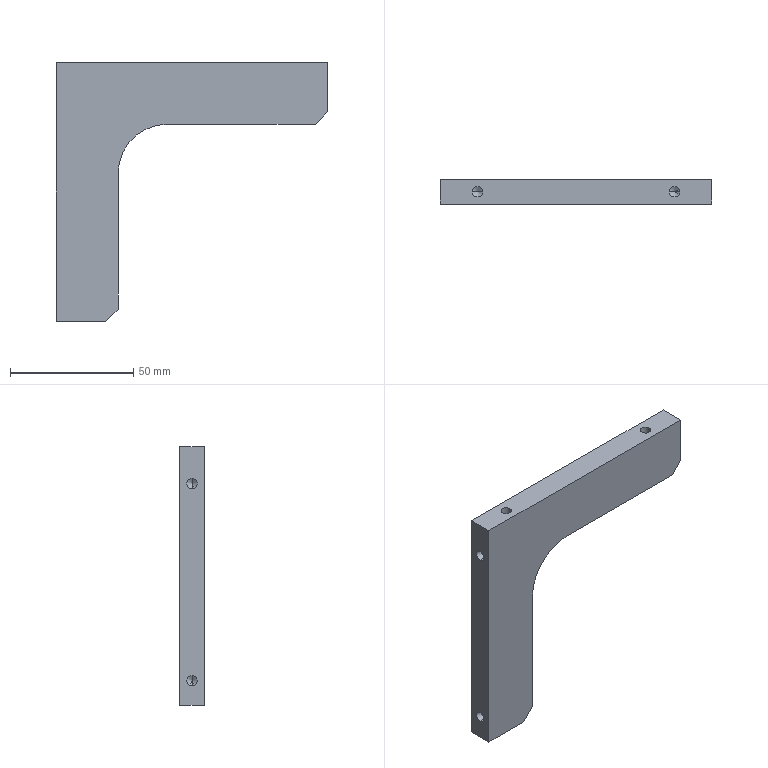Part | SolidWorks | features Chamfer 1, Extrusion 1, HoleWzd 1, ICE 1, MirrorPattern 1 | 1 solid | 27 faces | box 110 x 10 x 105 mm | volume 47398 mm3 | plane 10 | cylinder 9 | cone 8 | commonest cylinder face diameters 4.2 x8 40 x1
STEP:
#1=CARTESIAN_POINT('',(-42.1,0.,40.1));
#2=VERTEX_POINT('',#1);
#3=CARTESIAN_POINT('',(-37.9,0.,40.1));
#4=VERTEX_POINT('',#3);
#5=CARTESIAN_POINT('',(-40.,0.,40.1));
#6=DIRECTION('',(0.,0.,1.));
#7=DIRECTION('',(1.,0.,0.));
#8=AXIS2_PLACEMENT_3D('',#5,#6,#7);
#9=CIRCLE('',#8,2.1);
#10=EDGE_CURVE('',#2,#4,#9,.T.);
#11=ORIENTED_EDGE('',*,*,#10,.F.);
#12=CARTESIAN_POINT('',(-42.1,0.,52.5));
#13=VERTEX_POINT('',#12);
#14=CARTESIAN_POINT('',(-42.1,0.,52.5));
#15=DIRECTION('',(0.,0.,1.));
#16=VECTOR('',#15,1000.);
#17=LINE('',#14,#16);
#18=EDGE_CURVE('',#2,#13,#17,.T.);
#19=ORIENTED_EDGE('',*,*,#18,.T.);
#20=CARTESIAN_POINT('',(-37.9,0.,52.5));
#21=VERTEX_POINT('',#20);
#22=CARTESIAN_POINT('',(-40.,0.,52.5));
#23=DIRECTION('',(0.,0.,1.));
#24=DIRECTION('',(1.,0.,0.));
#25=AXIS2_PLACEMENT_3D('',#22,#23,#24);
#26=CIRCLE('',#25,2.1);
#27=EDGE_CURVE('',#13,#21,#26,.T.);
#28=ORIENTED_EDGE('',*,*,#27,.T.);
#29=CARTESIAN_POINT('',(-37.9,0.,52.5));
#30=DIRECTION('',(0.,0.,1.));
#31=VECTOR('',#30,1000.);
#32=LINE('',#29,#31);
#33=EDGE_CURVE('',#4,#21,#32,.T.);
#34=ORIENTED_EDGE('',*,*,#33,.F.);
#35=EDGE_LOOP('',(#11,#19,#28,#34));
#36=FACE_OUTER_BOUND('',#35,.T.);
#37=CARTESIAN_POINT('',(-40.,0.,52.5));
#38=DIRECTION('',(0.,0.,1.));
#39=DIRECTION('',(1.,0.,0.));
#40=AXIS2_PLACEMENT_3D('',#37,#38,#39);
#41=CYLINDRICAL_SURFACE('',#40,2.1);
#42=ADVANCED_FACE('',(#36),#41,.F.);
#43=CARTESIAN_POINT('',(-40.,0.,38.838));
#44=VERTEX_POINT('',#43);
#45=CARTESIAN_POINT('',(-37.9,0.,40.1));
#46=DIRECTION('',(0.8572,0.,0.515));
#47=VECTOR('',#46,1000.);
#48=LINE('',#45,#47);
#49=EDGE_CURVE('',#44,#4,#48,.T.);
#50=ORIENTED_EDGE('',*,*,#49,.F.);
#51=CARTESIAN_POINT('',(-42.1,0.,40.1));
#52=DIRECTION('',(-0.8572,0.,0.515));
#53=VECTOR('',#52,1000.);
#54=LINE('',#51,#53);
#55=EDGE_CURVE('',#44,#2,#54,.T.);
#56=ORIENTED_EDGE('',*,*,#55,.T.);
#57=ORIENTED_EDGE('',*,*,#10,.T.);
#58=EDGE_LOOP('',(#50,#56,#57));
#59=FACE_OUTER_BOUND('',#58,.T.);
#60=CARTESIAN_POINT('',(-40.,0.,40.1));
#61=DIRECTION('',(0.,0.,1.));
#62=DIRECTION('',(1.,0.,0.));
#63=AXIS2_PLACEMENT_3D('',#60,#61,#62);
#64=CONICAL_SURFACE('',#63,2.1,1.03);
#65=ADVANCED_FACE('',(#59),#64,.F.);
#66=CARTESIAN_POINT('',(37.9,0.,40.1));
#67=VERTEX_POINT('',#66);
#68=CARTESIAN_POINT('',(42.1,0.,40.1));
#69=VERTEX_POINT('',#68);
#70=CARTESIAN_POINT('',(40.,0.,40.1));
#71=DIRECTION('',(0.,0.,1.));
#72=DIRECTION('',(1.,0.,0.));
#73=AXIS2_PLACEMENT_3D('',#70,#71,#72);
#74=CIRCLE('',#73,2.1);
#75=EDGE_CURVE('',#67,#69,#74,.T.);
#76=ORIENTED_EDGE('',*,*,#75,.F.);
#77=CARTESIAN_POINT('',(37.9,0.,52.5));
#78=VERTEX_POINT('',#77);
#79=CARTESIAN_POINT('',(37.9,0.,52.5));
#80=DIRECTION('',(0.,0.,1.));
#81=VECTOR('',#80,1000.);
#82=LINE('',#79,#81);
#83=EDGE_CURVE('',#67,#78,#82,.T.);
#84=ORIENTED_EDGE('',*,*,#83,.T.);
#85=CARTESIAN_POINT('',(42.1,0.,52.5));
#86=VERTEX_POINT('',#85);
#87=CARTESIAN_POINT('',(40.,0.,52.5));
#88=DIRECTION('',(0.,0.,1.));
#89=DIRECTION('',(1.,0.,0.));
#90=AXIS2_PLACEMENT_3D('',#87,#88,#89);
#91=CIRCLE('',#90,2.1);
#92=EDGE_CURVE('',#78,#86,#91,.T.);
#93=ORIENTED_EDGE('',*,*,#92,.T.);
#94=CARTESIAN_POINT('',(42.1,0.,52.5));
#95=DIRECTION('',(0.,0.,1.));
#96=VECTOR('',#95,1000.);
#97=LINE('',#94,#96);
#98=EDGE_CURVE('',#69,#86,#97,.T.);
#99=ORIENTED_EDGE('',*,*,#98,.F.);
#100=EDGE_LOOP('',(#76,#84,#93,#99));
#101=FACE_OUTER_BOUND('',#100,.T.);
#102=CARTESIAN_POINT('',(40.,0.,52.5));
#103=DIRECTION('',(0.,0.,1.));
#104=DIRECTION('',(1.,0.,0.));
#105=AXIS2_PLACEMENT_3D('',#102,#103,#104);
#106=CYLINDRICAL_SURFACE('',#105,2.1);
#107=ADVANCED_FACE('',(#101),#106,.F.);
#108=CARTESIAN_POINT('',(40.,0.,38.838));
#109=VERTEX_POINT('',#108);
#110=CARTESIAN_POINT('',(42.1,0.,40.1));
#111=DIRECTION('',(0.8572,0.,0.515));
#112=VECTOR('',#111,1000.);
#113=LINE('',#110,#112);
#114=EDGE_CURVE('',#109,#69,#113,.T.);
#115=ORIENTED_EDGE('',*,*,#114,.F.);
#116=CARTESIAN_POINT('',(37.9,0.,40.1));
#117=DIRECTION('',(-0.8572,0.,0.515));
#118=VECTOR('',#117,1000.);
#119=LINE('',#116,#118);
#120=EDGE_CURVE('',#109,#67,#119,.T.);
#121=ORIENTED_EDGE('',*,*,#120,.T.);
#122=ORIENTED_EDGE('',*,*,#75,.T.);
#123=EDGE_LOOP('',(#115,#121,#122));
#124=FACE_OUTER_BOUND('',#123,.T.);
#125=CARTESIAN_POINT('',(40.,0.,40.1));
#126=DIRECTION('',(0.,0.,1.));
#127=DIRECTION('',(1.,0.,0.));
#128=AXIS2_PLACEMENT_3D('',#125,#126,#127);
#129=CONICAL_SURFACE('',#128,2.1,1.03);
#130=ADVANCED_FACE('',(#124),#129,.F.);
#131=CARTESIAN_POINT('',(-42.6,0.,35.4));
#132=VERTEX_POINT('',#131);
#133=CARTESIAN_POINT('',(-42.6,0.,39.6));
#134=VERTEX_POINT('',#133);
#135=CARTESIAN_POINT('',(-42.6,0.,37.5));
#136=DIRECTION('',(-1.,0.,0.));
#137=DIRECTION('',(0.,0.,1.));
#138=AXIS2_PLACEMENT_3D('',#135,#136,#137);
#139=CIRCLE('',#138,2.1);
#140=EDGE_CURVE('',#132,#134,#139,.T.);
#141=ORIENTED_EDGE('',*,*,#140,.F.);
#142=CARTESIAN_POINT('',(-55.,0.,35.4));
#143=VERTEX_POINT('',#142);
#144=CARTESIAN_POINT('',(-55.,0.,35.4));
#145=DIRECTION('',(-1.,0.,0.));
#146=VECTOR('',#145,1000.);
#147=LINE('',#144,#146);
#148=EDGE_CURVE('',#132,#143,#147,.T.);
#149=ORIENTED_EDGE('',*,*,#148,.T.);
#150=CARTESIAN_POINT('',(-55.,0.,39.6));
#151=VERTEX_POINT('',#150);
#152=CARTESIAN_POINT('',(-55.,0.,37.5));
#153=DIRECTION('',(-1.,0.,0.));
#154=DIRECTION('',(0.,0.,1.));
#155=AXIS2_PLACEMENT_3D('',#152,#153,#154);
#156=CIRCLE('',#155,2.1);
#157=EDGE_CURVE('',#143,#151,#156,.T.);
#158=ORIENTED_EDGE('',*,*,#157,.T.);
#159=CARTESIAN_POINT('',(-55.,0.,39.6));
#160=DIRECTION('',(-1.,0.,0.));
#161=VECTOR('',#160,1000.);
#162=LINE('',#159,#161);
#163=EDGE_CURVE('',#134,#151,#162,.T.);
#164=ORIENTED_EDGE('',*,*,#163,.F.);
#165=EDGE_LOOP('',(#141,#149,#158,#164));
#166=FACE_OUTER_BOUND('',#165,.T.);
#167=CARTESIAN_POINT('',(-55.,0.,37.5));
#168=DIRECTION('',(-1.,0.,0.));
#169=DIRECTION('',(0.,0.,1.));
#170=AXIS2_PLACEMENT_3D('',#167,#168,#169);
#171=CYLINDRICAL_SURFACE('',#170,2.1);
#172=ADVANCED_FACE('',(#166),#171,.F.);
#173=CARTESIAN_POINT('',(-41.338,0.,37.5));
#174=VERTEX_POINT('',#173);
#175=CARTESIAN_POINT('',(-42.6,0.,39.6));
#176=DIRECTION('',(-0.515,0.,0.8572));
#177=VECTOR('',#176,1000.);
#178=LINE('',#175,#177);
#179=EDGE_CURVE('',#174,#134,#178,.T.);
#180=ORIENTED_EDGE('',*,*,#179,.F.);
#181=CARTESIAN_POINT('',(-42.6,0.,35.4));
#182=DIRECTION('',(-0.515,0.,-0.8572));
#183=VECTOR('',#182,1000.);
#184=LINE('',#181,#183);
#185=EDGE_CURVE('',#174,#132,#184,.T.);
#186=ORIENTED_EDGE('',*,*,#185,.T.);
#187=ORIENTED_EDGE('',*,*,#140,.T.);
#188=EDGE_LOOP('',(#180,#186,#187));
#189=FACE_OUTER_BOUND('',#188,.T.);
#190=CARTESIAN_POINT('',(-42.6,0.,37.5));
#191=DIRECTION('',(-1.,0.,0.));
#192=DIRECTION('',(0.,0.,1.));
#193=AXIS2_PLACEMENT_3D('',#190,#191,#192);
#194=CONICAL_SURFACE('',#193,2.1,1.03);
#195=ADVANCED_FACE('',(#189),#194,.F.);
#196=CARTESIAN_POINT('',(-42.6,0.,-44.6));
#197=VERTEX_POINT('',#196);
#198=CARTESIAN_POINT('',(-42.6,0.,-40.4));
#199=VERTEX_POINT('',#198);
#200=CARTESIAN_POINT('',(-42.6,0.,-42.5));
#201=DIRECTION('',(-1.,0.,0.));
#202=DIRECTION('',(0.,0.,1.));
#203=AXIS2_PLACEMENT_3D('',#200,#201,#202);
#204=CIRCLE('',#203,2.1);
#205=EDGE_CURVE('',#197,#199,#204,.T.);
#206=ORIENTED_EDGE('',*,*,#205,.F.);
#207=CARTESIAN_POINT('',(-55.,0.,-44.6));
#208=VERTEX_POINT('',#207);
#209=CARTESIAN_POINT('',(-55.,0.,-44.6));
#210=DIRECTION('',(-1.,0.,0.));
#211=VECTOR('',#210,1000.);
#212=LINE('',#209,#211);
#213=EDGE_CURVE('',#197,#208,#212,.T.);
#214=ORIENTED_EDGE('',*,*,#213,.T.);
#215=CARTESIAN_POINT('',(-55.,0.,-40.4));
#216=VERTEX_POINT('',#215);
#217=CARTESIAN_POINT('',(-55.,0.,-42.5));
#218=DIRECTION('',(-1.,0.,0.));
#219=DIRECTION('',(0.,0.,1.));
#220=AXIS2_PLACEMENT_3D('',#217,#218,#219);
#221=CIRCLE('',#220,2.1);
#222=EDGE_CURVE('',#208,#216,#221,.T.);
#223=ORIENTED_EDGE('',*,*,#222,.T.);
#224=CARTESIAN_POINT('',(-55.,0.,-40.4));
#225=DIRECTION('',(-1.,0.,0.));
#226=VECTOR('',#225,1000.);
#227=LINE('',#224,#226);
#228=EDGE_CURVE('',#199,#216,#227,.T.);
#229=ORIENTED_EDGE('',*,*,#228,.F.);
#230=EDGE_LOOP('',(#206,#214,#223,#229));
#231=FACE_OUTER_BOUND('',#230,.T.);
#232=CARTESIAN_POINT('',(-55.,0.,-42.5));
#233=DIRECTION('',(-1.,0.,0.));
#234=DIRECTION('',(0.,0.,1.));
#235=AXIS2_PLACEMENT_3D('',#232,#233,#234);
#236=CYLINDRICAL_SURFACE('',#235,2.1);
#237=ADVANCED_FACE('',(#231),#236,.F.);
#238=CARTESIAN_POINT('',(-41.338,0.,-42.5));
#239=VERTEX_POINT('',#238);
#240=CARTESIAN_POINT('',(-42.6,0.,-40.4));
#241=DIRECTION('',(-0.515,0.,0.8572));
#242=VECTOR('',#241,1000.);
#243=LINE('',#240,#242);
#244=EDGE_CURVE('',#239,#199,#243,.T.);
#245=ORIENTED_EDGE('',*,*,#244,.F.);
#246=CARTESIAN_POINT('',(-42.6,0.,-44.6));
#247=DIRECTION('',(-0.515,0.,-0.8572));
#248=VECTOR('',#247,1000.);
#249=LINE('',#246,#248);
#250=EDGE_CURVE('',#239,#197,#249,.T.);
#251=ORIENTED_EDGE('',*,*,#250,.T.);
#252=ORIENTED_EDGE('',*,*,#205,.T.);
#253=EDGE_LOOP('',(#245,#251,#252));
#254=FACE_OUTER_BOUND('',#253,.T.);
#255=CARTESIAN_POINT('',(-42.6,0.,-42.5));
#256=DIRECTION('',(-1.,0.,0.));
#257=DIRECTION('',(0.,0.,1.));
#258=AXIS2_PLACEMENT_3D('',#255,#256,#257);
#259=CONICAL_SURFACE('',#258,2.1,1.03);
#260=ADVANCED_FACE('',(#254),#259,.F.);
#261=CARTESIAN_POINT('',(55.,-5.,52.5));
#262=VERTEX_POINT('',#261);
#263=CARTESIAN_POINT('',(55.,-5.,32.5));
#264=VERTEX_POINT('',#263);
#265=CARTESIAN_POINT('',(55.,-5.,52.5));
#266=DIRECTION('',(0.,0.,-1.));
#267=VECTOR('',#266,1000.);
#268=LINE('',#265,#267);
#269=EDGE_CURVE('',#262,#264,#268,.T.);
#270=ORIENTED_EDGE('',*,*,#269,.T.);
#271=CARTESIAN_POINT('',(55.,5.,32.5));
#272=VERTEX_POINT('',#271);
#273=CARTESIAN_POINT('',(55.,5.,32.5));
#274=DIRECTION('',(0.,1.,0.));
#275=VECTOR('',#274,1000.);
#276=LINE('',#273,#275);
#277=EDGE_CURVE('',#264,#272,#276,.T.);
#278=ORIENTED_EDGE('',*,*,#277,.T.);
#279=CARTESIAN_POINT('',(55.,5.,52.5));
#280=VERTEX_POINT('',#279);
#281=CARTESIAN_POINT('',(55.,5.,52.5));
#282=DIRECTION('',(0.,0.,-1.));
#283=VECTOR('',#282,1000.);
#284=LINE('',#281,#283);
#285=EDGE_CURVE('',#280,#272,#284,.T.);
#286=ORIENTED_EDGE('',*,*,#285,.F.);
#287=CARTESIAN_POINT('',(55.,5.,52.5));
#288=DIRECTION('',(0.,-1.,0.));
#289=VECTOR('',#288,1000.);
#290=LINE('',#287,#289);
#291=EDGE_CURVE('',#280,#262,#290,.T.);
#292=ORIENTED_EDGE('',*,*,#291,.T.);
#293=EDGE_LOOP('',(#270,#278,#286,#292));
#294=FACE_OUTER_BOUND('',#293,.T.);
#295=CARTESIAN_POINT('',(55.,5.,52.5));
#296=DIRECTION('',(-1.,0.,0.));
#297=DIRECTION('',(0.,0.,1.));
#298=AXIS2_PLACEMENT_3D('',#295,#296,#297);
#299=PLANE('',#298);
#300=ADVANCED_FACE('',(#294),#299,.F.);
#301=CARTESIAN_POINT('',(-35.,5.,-52.5));
#302=VERTEX_POINT('',#301);
#303=CARTESIAN_POINT('',(-55.,5.,-52.5));
#304=VERTEX_POINT('',#303);
#305=CARTESIAN_POINT('',(-55.,5.,-52.5));
#306=DIRECTION('',(-1.,0.,0.));
#307=VECTOR('',#306,1000.);
#308=LINE('',#305,#307);
#309=EDGE_CURVE('',#302,#304,#308,.T.);
#310=ORIENTED_EDGE('',*,*,#309,.F.);
#311=CARTESIAN_POINT('',(-35.,-5.,-52.5));
#312=VERTEX_POINT('',#311);
#313=CARTESIAN_POINT('',(-35.,5.,-52.5));
#314=DIRECTION('',(0.,-1.,0.));
#315=VECTOR('',#314,1000.);
#316=LINE('',#313,#315);
#317=EDGE_CURVE('',#302,#312,#316,.T.);
#318=ORIENTED_EDGE('',*,*,#317,.T.);
#319=CARTESIAN_POINT('',(-55.,-5.,-52.5));
#320=VERTEX_POINT('',#319);
#321=CARTESIAN_POINT('',(-55.,-5.,-52.5));
#322=DIRECTION('',(-1.,0.,0.));
#323=VECTOR('',#322,1000.);
#324=LINE('',#321,#323);
#325=EDGE_CURVE('',#312,#320,#324,.T.);
#326=ORIENTED_EDGE('',*,*,#325,.T.);
#327=CARTESIAN_POINT('',(-55.,5.,-52.5));
#328=DIRECTION('',(0.,-1.,0.));
#329=VECTOR('',#328,1000.);
#330=LINE('',#327,#329);
#331=EDGE_CURVE('',#304,#320,#330,.T.);
#332=ORIENTED_EDGE('',*,*,#331,.F.);
#333=EDGE_LOOP('',(#310,#318,#326,#332));
#334=FACE_OUTER_BOUND('',#333,.T.);
#335=CARTESIAN_POINT('',(-55.,5.,-52.5));
#336=DIRECTION('',(0.,0.,1.));
#337=DIRECTION('',(1.,0.,0.));
#338=AXIS2_PLACEMENT_3D('',#335,#336,#337);
#339=PLANE('',#338);
#340=ADVANCED_FACE('',(#334),#339,.F.);
#341=CARTESIAN_POINT('',(-55.,0.,37.5));
#342=DIRECTION('',(-1.,0.,0.));
#343=DIRECTION('',(0.,0.,1.));
#344=AXIS2_PLACEMENT_3D('',#341,#342,#343);
#345=CIRCLE('',#344,2.1);
#346=EDGE_CURVE('',#151,#143,#345,.T.);
#347=ORIENTED_EDGE('',*,*,#346,.F.);
#348=ORIENTED_EDGE('',*,*,#157,.F.);
#349=EDGE_LOOP('',(#347,#348));
#350=FACE_BOUND('',#349,.T.);
#351=CARTESIAN_POINT('',(-55.,0.,-42.5));
#352=DIRECTION('',(-1.,0.,0.));
#353=DIRECTION('',(0.,0.,1.));
#354=AXIS2_PLACEMENT_3D('',#351,#352,#353);
#355=CIRCLE('',#354,2.1);
#356=EDGE_CURVE('',#216,#208,#355,.T.);
#357=ORIENTED_EDGE('',*,*,#356,.F.);
#358=ORIENTED_EDGE('',*,*,#222,.F.);
#359=EDGE_LOOP('',(#357,#358));
#360=FACE_BOUND('',#359,.T.);
#361=CARTESIAN_POINT('',(-55.,-5.,52.5));
#362=VERTEX_POINT('',#361);
#363=CARTESIAN_POINT('',(-55.,-5.,52.5));
#364=DIRECTION('',(0.,0.,1.));
#365=VECTOR('',#364,1000.);
#366=LINE('',#363,#365);
#367=EDGE_CURVE('',#320,#362,#366,.T.);
#368=ORIENTED_EDGE('',*,*,#367,.T.);
#369=CARTESIAN_POINT('',(-55.,5.,52.5));
#370=VERTEX_POINT('',#369);
#371=CARTESIAN_POINT('',(-55.,5.,52.5));
#372=DIRECTION('',(0.,-1.,0.));
#373=VECTOR('',#372,1000.);
#374=LINE('',#371,#373);
#375=EDGE_CURVE('',#370,#362,#374,.T.);
#376=ORIENTED_EDGE('',*,*,#375,.F.);
#377=CARTESIAN_POINT('',(-55.,5.,52.5));
#378=DIRECTION('',(0.,0.,1.));
#379=VECTOR('',#378,1000.);
#380=LINE('',#377,#379);
#381=EDGE_CURVE('',#304,#370,#380,.T.);
#382=ORIENTED_EDGE('',*,*,#381,.F.);
#383=ORIENTED_EDGE('',*,*,#331,.T.);
#384=EDGE_LOOP('',(#368,#376,#382,#383));
#385=FACE_OUTER_BOUND('',#384,.T.);
#386=CARTESIAN_POINT('',(-55.,5.,52.5));
#387=DIRECTION('',(1.,0.,0.));
#388=DIRECTION('',(0.,0.,-1.));
#389=AXIS2_PLACEMENT_3D('',#386,#387,#388);
#390=PLANE('',#389);
#391=ADVANCED_FACE('',(#350,#360,#385),#390,.F.);
#392=CARTESIAN_POINT('',(-40.,0.,52.5));
#393=DIRECTION('',(0.,0.,1.));
#394=DIRECTION('',(1.,0.,0.));
#395=AXIS2_PLACEMENT_3D('',#392,#393,#394);
#396=CIRCLE('',#395,2.1);
#397=EDGE_CURVE('',#21,#13,#396,.T.);
#398=ORIENTED_EDGE('',*,*,#397,.F.);
#399=ORIENTED_EDGE('',*,*,#27,.F.);
#400=EDGE_LOOP('',(#398,#399));
#401=FACE_BOUND('',#400,.T.);
#402=CARTESIAN_POINT('',(40.,0.,52.5));
#403=DIRECTION('',(0.,0.,1.));
#404=DIRECTION('',(1.,0.,0.));
#405=AXIS2_PLACEMENT_3D('',#402,#403,#404);
#406=CIRCLE('',#405,2.1);
#407=EDGE_CURVE('',#86,#78,#406,.T.);
#408=ORIENTED_EDGE('',*,*,#407,.F.);
#409=ORIENTED_EDGE('',*,*,#92,.F.);
#410=EDGE_LOOP('',(#408,#409));
#411=FACE_BOUND('',#410,.T.);
#412=CARTESIAN_POINT('',(-55.,-5.,52.5));
#413=DIRECTION('',(1.,0.,0.));
#414=VECTOR('',#413,1000.);
#415=LINE('',#412,#414);
#416=EDGE_CURVE('',#362,#262,#415,.T.);
#417=ORIENTED_EDGE('',*,*,#416,.T.);
#418=ORIENTED_EDGE('',*,*,#291,.F.);
#419=CARTESIAN_POINT('',(-55.,5.,52.5));
#420=DIRECTION('',(1.,0.,0.));
#421=VECTOR('',#420,1000.);
#422=LINE('',#419,#421);
#423=EDGE_CURVE('',#370,#280,#422,.T.);
#424=ORIENTED_EDGE('',*,*,#423,.F.);
#425=ORIENTED_EDGE('',*,*,#375,.T.);
#426=EDGE_LOOP('',(#417,#418,#424,#425));
#427=FACE_OUTER_BOUND('',#426,.T.);
#428=CARTESIAN_POINT('',(-55.,5.,52.5));
#429=DIRECTION('',(0.,0.,-1.));
#430=DIRECTION('',(-1.,0.,0.));
#431=AXIS2_PLACEMENT_3D('',#428,#429,#430);
#432=PLANE('',#431);
#433=ADVANCED_FACE('',(#401,#411,#427),#432,.F.);
#434=CARTESIAN_POINT('',(-30.,5.,-47.5));
#435=VERTEX_POINT('',#434);
#436=CARTESIAN_POINT('',(-30.,5.,7.5));
#437=VERTEX_POINT('',#436);
#438=CARTESIAN_POINT('',(-30.,5.,-52.5));
#439=DIRECTION('',(0.,0.,1.));
#440=VECTOR('',#439,1000.);
#441=LINE('',#438,#440);
#442=EDGE_CURVE('',#435,#437,#441,.T.);
#443=ORIENTED_EDGE('',*,*,#442,.F.);
#444=CARTESIAN_POINT('',(-30.,5.,-47.5));
#445=DIRECTION('',(-0.7071,0.,-0.7071));
#446=VECTOR('',#445,1000.);
#447=LINE('',#444,#446);
#448=EDGE_CURVE('',#435,#302,#447,.T.);
#449=ORIENTED_EDGE('',*,*,#448,.T.);
#450=ORIENTED_EDGE('',*,*,#309,.T.);
#451=ORIENTED_EDGE('',*,*,#381,.T.);
#452=ORIENTED_EDGE('',*,*,#423,.T.);
#453=ORIENTED_EDGE('',*,*,#285,.T.);
#454=CARTESIAN_POINT('',(50.,5.,27.5));
#455=VERTEX_POINT('',#454);
#456=CARTESIAN_POINT('',(55.,5.,32.5));
#457=DIRECTION('',(-0.7071,0.,-0.7071));
#458=VECTOR('',#457,1000.);
#459=LINE('',#456,#458);
#460=EDGE_CURVE('',#272,#455,#459,.T.);
#461=ORIENTED_EDGE('',*,*,#460,.T.);
#462=CARTESIAN_POINT('',(-10.,5.,27.5));
#463=VERTEX_POINT('',#462);
#464=CARTESIAN_POINT('',(55.,5.,27.5));
#465=DIRECTION('',(1.,0.,0.));
#466=VECTOR('',#465,1000.);
#467=LINE('',#464,#466);
#468=EDGE_CURVE('',#463,#455,#467,.T.);
#469=ORIENTED_EDGE('',*,*,#468,.F.);
#470=CARTESIAN_POINT('',(-10.,5.,7.5));
#471=DIRECTION('',(0.,1.,0.));
#472=DIRECTION('',(0.,0.,-1.));
#473=AXIS2_PLACEMENT_3D('',#470,#471,#472);
#474=CIRCLE('',#473,20.);
#475=EDGE_CURVE('',#437,#463,#474,.T.);
#476=ORIENTED_EDGE('',*,*,#475,.F.);
#477=EDGE_LOOP('',(#443,#449,#450,#451,#452,#453,#461,#469,#476));
#478=FACE_OUTER_BOUND('',#477,.T.);
#479=CARTESIAN_POINT('',(0.,5.,0.));
#480=DIRECTION('',(0.,-1.,0.));
#481=DIRECTION('',(0.,0.,-1.));
#482=AXIS2_PLACEMENT_3D('',#479,#480,#481);
#483=PLANE('',#482);
#484=ADVANCED_FACE('',(#478),#483,.F.);
#485=ORIENTED_EDGE('',*,*,#325,.F.);
#486=CARTESIAN_POINT('',(-30.,-5.,-47.5));
#487=VERTEX_POINT('',#486);
#488=CARTESIAN_POINT('',(8.75,-5.,-8.75));
#489=DIRECTION('',(0.7071,0.,0.7071));
#490=VECTOR('',#489,1000.);
#491=LINE('',#488,#490);
#492=EDGE_CURVE('',#312,#487,#491,.T.);
#493=ORIENTED_EDGE('',*,*,#492,.T.);
#494=CARTESIAN_POINT('',(-30.,-5.,7.5));
#495=VERTEX_POINT('',#494);
#496=CARTESIAN_POINT('',(-30.,-5.,-52.5));
#497=DIRECTION('',(0.,0.,1.));
#498=VECTOR('',#497,1000.);
#499=LINE('',#496,#498);
#500=EDGE_CURVE('',#487,#495,#499,.T.);
#501=ORIENTED_EDGE('',*,*,#500,.T.);
#502=CARTESIAN_POINT('',(-10.,-5.,27.5));
#503=VERTEX_POINT('',#502);
#504=CARTESIAN_POINT('',(-10.,-5.,7.5));
#505=DIRECTION('',(0.,1.,0.));
#506=DIRECTION('',(0.,0.,-1.));
#507=AXIS2_PLACEMENT_3D('',#504,#505,#506);
#508=CIRCLE('',#507,20.);
#509=EDGE_CURVE('',#495,#503,#508,.T.);
#510=ORIENTED_EDGE('',*,*,#509,.T.);
#511=CARTESIAN_POINT('',(50.,-5.,27.5));
#512=VERTEX_POINT('',#511);
#513=CARTESIAN_POINT('',(55.,-5.,27.5));
#514=DIRECTION('',(1.,0.,0.));
#515=VECTOR('',#514,1000.);
#516=LINE('',#513,#515);
#517=EDGE_CURVE('',#503,#512,#516,.T.);
#518=ORIENTED_EDGE('',*,*,#517,.T.);
#519=CARTESIAN_POINT('',(11.25,-5.,-11.25));
#520=DIRECTION('',(0.7071,0.,0.7071));
#521=VECTOR('',#520,1000.);
#522=LINE('',#519,#521);
#523=EDGE_CURVE('',#512,#264,#522,.T.);
#524=ORIENTED_EDGE('',*,*,#523,.T.);
#525=ORIENTED_EDGE('',*,*,#269,.F.);
#526=ORIENTED_EDGE('',*,*,#416,.F.);
#527=ORIENTED_EDGE('',*,*,#367,.F.);
#528=EDGE_LOOP('',(#485,#493,#501,#510,#518,#524,#525,#526,#527));
#529=FACE_OUTER_BOUND('',#528,.T.);
#530=CARTESIAN_POINT('',(0.,-5.,0.));
#531=DIRECTION('',(0.,-1.,0.));
#532=DIRECTION('',(0.,0.,-1.));
#533=AXIS2_PLACEMENT_3D('',#530,#531,#532);
#534=PLANE('',#533);
#535=ADVANCED_FACE('',(#529),#534,.T.);
#536=ORIENTED_EDGE('',*,*,#500,.F.);
#537=CARTESIAN_POINT('',(-30.,-121.726,-47.5));
#538=DIRECTION('',(0.,1.,0.));
#539=VECTOR('',#538,1000.);
#540=LINE('',#537,#539);
#541=EDGE_CURVE('',#487,#435,#540,.T.);
#542=ORIENTED_EDGE('',*,*,#541,.T.);
#543=ORIENTED_EDGE('',*,*,#442,.T.);
#544=CARTESIAN_POINT('',(-30.,-121.726,7.5));
#545=DIRECTION('',(0.,1.,0.));
#546=VECTOR('',#545,1000.);
#547=LINE('',#544,#546);
#548=EDGE_CURVE('',#495,#437,#547,.T.);
#549=ORIENTED_EDGE('',*,*,#548,.F.);
#550=EDGE_LOOP('',(#536,#542,#543,#549));
#551=FACE_OUTER_BOUND('',#550,.T.);
#552=CARTESIAN_POINT('',(-30.,-121.726,-52.5));
#553=DIRECTION('',(-1.,0.,0.));
#554=DIRECTION('',(0.,0.,1.));
#555=AXIS2_PLACEMENT_3D('',#552,#553,#554);
#556=PLANE('',#555);
#557=ADVANCED_FACE('',(#551),#556,.F.);
#558=ORIENTED_EDGE('',*,*,#548,.T.);
#559=ORIENTED_EDGE('',*,*,#475,.T.);
#560=CARTESIAN_POINT('',(-10.,-121.726,27.5));
#561=DIRECTION('',(0.,1.,0.));
#562=VECTOR('',#561,1000.);
#563=LINE('',#560,#562);
#564=EDGE_CURVE('',#503,#463,#563,.T.);
#565=ORIENTED_EDGE('',*,*,#564,.F.);
#566=ORIENTED_EDGE('',*,*,#509,.F.);
#567=EDGE_LOOP('',(#558,#559,#565,#566));
#568=FACE_OUTER_BOUND('',#567,.T.);
#569=CARTESIAN_POINT('',(-10.,-121.726,7.5));
#570=DIRECTION('',(0.,1.,0.));
#571=DIRECTION('',(0.,0.,1.));
#572=AXIS2_PLACEMENT_3D('',#569,#570,#571);
#573=CYLINDRICAL_SURFACE('',#572,20.);
#574=ADVANCED_FACE('',(#568),#573,.F.);
#575=ORIENTED_EDGE('',*,*,#468,.T.);
#576=CARTESIAN_POINT('',(50.,-121.726,27.5));
#577=DIRECTION('',(0.,-1.,0.));
#578=VECTOR('',#577,1000.);
#579=LINE('',#576,#578);
#580=EDGE_CURVE('',#455,#512,#579,.T.);
#581=ORIENTED_EDGE('',*,*,#580,.T.);
#582=ORIENTED_EDGE('',*,*,#517,.F.);
#583=ORIENTED_EDGE('',*,*,#564,.T.);
#584=EDGE_LOOP('',(#575,#581,#582,#583));
#585=FACE_OUTER_BOUND('',#584,.T.);
#586=CARTESIAN_POINT('',(55.,-121.726,27.5));
#587=DIRECTION('',(0.,0.,1.));
#588=DIRECTION('',(1.,0.,0.));
#589=AXIS2_PLACEMENT_3D('',#586,#587,#588);
#590=PLANE('',#589);
#591=ADVANCED_FACE('',(#585),#590,.F.);
#592=ORIENTED_EDGE('',*,*,#492,.F.);
#593=ORIENTED_EDGE('',*,*,#317,.F.);
#594=ORIENTED_EDGE('',*,*,#448,.F.);
#595=ORIENTED_EDGE('',*,*,#541,.F.);
#596=EDGE_LOOP('',(#592,#593,#594,#595));
#597=FACE_OUTER_BOUND('',#596,.T.);
#598=CARTESIAN_POINT('',(-30.,-121.726,-47.5));
#599=DIRECTION('',(-0.7071,0.,0.7071));
#600=DIRECTION('',(0.,1.,0.));
#601=AXIS2_PLACEMENT_3D('',#598,#599,#600);
#602=PLANE('',#601);
#603=ADVANCED_FACE('',(#597),#602,.F.);
#604=ORIENTED_EDGE('',*,*,#523,.F.);
#605=ORIENTED_EDGE('',*,*,#580,.F.);
#606=ORIENTED_EDGE('',*,*,#460,.F.);
#607=ORIENTED_EDGE('',*,*,#277,.F.);
#608=EDGE_LOOP('',(#604,#605,#606,#607));
#609=FACE_OUTER_BOUND('',#608,.T.);
#610=CARTESIAN_POINT('',(55.,5.,32.5));
#611=DIRECTION('',(-0.7071,0.,0.7071));
#612=DIRECTION('',(0.,1.,0.));
#613=AXIS2_PLACEMENT_3D('',#610,#611,#612);
#614=PLANE('',#613);
#615=ADVANCED_FACE('',(#609),#614,.F.);
#616=ORIENTED_EDGE('',*,*,#250,.F.);
#617=ORIENTED_EDGE('',*,*,#244,.T.);
#618=CARTESIAN_POINT('',(-42.6,0.,-42.5));
#619=DIRECTION('',(-1.,0.,0.));
#620=DIRECTION('',(0.,0.,1.));
#621=AXIS2_PLACEMENT_3D('',#618,#619,#620);
#622=CIRCLE('',#621,2.1);
#623=EDGE_CURVE('',#199,#197,#622,.T.);
#624=ORIENTED_EDGE('',*,*,#623,.T.);
#625=EDGE_LOOP('',(#616,#617,#624));
#626=FACE_OUTER_BOUND('',#625,.T.);
#627=CARTESIAN_POINT('',(-42.6,0.,-42.5));
#628=DIRECTION('',(-1.,0.,0.));
#629=DIRECTION('',(0.,0.,1.));
#630=AXIS2_PLACEMENT_3D('',#627,#628,#629);
#631=CONICAL_SURFACE('',#630,2.1,1.03);
#632=ADVANCED_FACE('',(#626),#631,.F.);
#633=ORIENTED_EDGE('',*,*,#213,.F.);
#634=ORIENTED_EDGE('',*,*,#623,.F.);
#635=ORIENTED_EDGE('',*,*,#228,.T.);
#636=ORIENTED_EDGE('',*,*,#356,.T.);
#637=EDGE_LOOP('',(#633,#634,#635,#636));
#638=FACE_OUTER_BOUND('',#637,.T.);
#639=CARTESIAN_POINT('',(-55.,0.,-42.5));
#640=DIRECTION('',(-1.,0.,0.));
#641=DIRECTION('',(0.,0.,1.));
#642=AXIS2_PLACEMENT_3D('',#639,#640,#641);
#643=CYLINDRICAL_SURFACE('',#642,2.1);
#644=ADVANCED_FACE('',(#638),#643,.F.);
#645=ORIENTED_EDGE('',*,*,#185,.F.);
#646=ORIENTED_EDGE('',*,*,#179,.T.);
#647=CARTESIAN_POINT('',(-42.6,0.,37.5));
#648=DIRECTION('',(-1.,0.,0.));
#649=DIRECTION('',(0.,0.,1.));
#650=AXIS2_PLACEMENT_3D('',#647,#648,#649);
#651=CIRCLE('',#650,2.1);
#652=EDGE_CURVE('',#134,#132,#651,.T.);
#653=ORIENTED_EDGE('',*,*,#652,.T.);
#654=EDGE_LOOP('',(#645,#646,#653));
#655=FACE_OUTER_BOUND('',#654,.T.);
#656=CARTESIAN_POINT('',(-42.6,0.,37.5));
#657=DIRECTION('',(-1.,0.,0.));
#658=DIRECTION('',(0.,0.,1.));
#659=AXIS2_PLACEMENT_3D('',#656,#657,#658);
#660=CONICAL_SURFACE('',#659,2.1,1.03);
#661=ADVANCED_FACE('',(#655),#660,.F.);
#662=ORIENTED_EDGE('',*,*,#148,.F.);
#663=ORIENTED_EDGE('',*,*,#652,.F.);
#664=ORIENTED_EDGE('',*,*,#163,.T.);
#665=ORIENTED_EDGE('',*,*,#346,.T.);
#666=EDGE_LOOP('',(#662,#663,#664,#665));
#667=FACE_OUTER_BOUND('',#666,.T.);
#668=CARTESIAN_POINT('',(-55.,0.,37.5));
#669=DIRECTION('',(-1.,0.,0.));
#670=DIRECTION('',(0.,0.,1.));
#671=AXIS2_PLACEMENT_3D('',#668,#669,#670);
#672=CYLINDRICAL_SURFACE('',#671,2.1);
#673=ADVANCED_FACE('',(#667),#672,.F.);
#674=ORIENTED_EDGE('',*,*,#120,.F.);
#675=ORIENTED_EDGE('',*,*,#114,.T.);
#676=CARTESIAN_POINT('',(40.,0.,40.1));
#677=DIRECTION('',(0.,0.,1.));
#678=DIRECTION('',(1.,0.,0.));
#679=AXIS2_PLACEMENT_3D('',#676,#677,#678);
#680=CIRCLE('',#679,2.1);
#681=EDGE_CURVE('',#69,#67,#680,.T.);
#682=ORIENTED_EDGE('',*,*,#681,.T.);
#683=EDGE_LOOP('',(#674,#675,#682));
#684=FACE_OUTER_BOUND('',#683,.T.);
#685=CARTESIAN_POINT('',(40.,0.,40.1));
#686=DIRECTION('',(0.,0.,1.));
#687=DIRECTION('',(1.,0.,0.));
#688=AXIS2_PLACEMENT_3D('',#685,#686,#687);
#689=CONICAL_SURFACE('',#688,2.1,1.03);
#690=ADVANCED_FACE('',(#684),#689,.F.);
#691=ORIENTED_EDGE('',*,*,#83,.F.);
#692=ORIENTED_EDGE('',*,*,#681,.F.);
#693=ORIENTED_EDGE('',*,*,#98,.T.);
#694=ORIENTED_EDGE('',*,*,#407,.T.);
#695=EDGE_LOOP('',(#691,#692,#693,#694));
#696=FACE_OUTER_BOUND('',#695,.T.);
#697=CARTESIAN_POINT('',(40.,0.,52.5));
#698=DIRECTION('',(0.,0.,1.));
#699=DIRECTION('',(1.,0.,0.));
#700=AXIS2_PLACEMENT_3D('',#697,#698,#699);
#701=CYLINDRICAL_SURFACE('',#700,2.1);
#702=ADVANCED_FACE('',(#696),#701,.F.);
#703=ORIENTED_EDGE('',*,*,#55,.F.);
#704=ORIENTED_EDGE('',*,*,#49,.T.);
#705=CARTESIAN_POINT('',(-40.,0.,40.1));
#706=DIRECTION('',(0.,0.,1.));
#707=DIRECTION('',(1.,0.,0.));
#708=AXIS2_PLACEMENT_3D('',#705,#706,#707);
#709=CIRCLE('',#708,2.1);
#710=EDGE_CURVE('',#4,#2,#709,.T.);
#711=ORIENTED_EDGE('',*,*,#710,.T.);
#712=EDGE_LOOP('',(#703,#704,#711));
#713=FACE_OUTER_BOUND('',#712,.T.);
#714=CARTESIAN_POINT('',(-40.,0.,40.1));
#715=DIRECTION('',(0.,0.,1.));
#716=DIRECTION('',(1.,0.,0.));
#717=AXIS2_PLACEMENT_3D('',#714,#715,#716);
#718=CONICAL_SURFACE('',#717,2.1,1.03);
#719=ADVANCED_FACE('',(#713),#718,.F.);
#720=ORIENTED_EDGE('',*,*,#18,.F.);
#721=ORIENTED_EDGE('',*,*,#710,.F.);
#722=ORIENTED_EDGE('',*,*,#33,.T.);
#723=ORIENTED_EDGE('',*,*,#397,.T.);
#724=EDGE_LOOP('',(#720,#721,#722,#723));
#725=FACE_OUTER_BOUND('',#724,.T.);
#726=CARTESIAN_POINT('',(-40.,0.,52.5));
#727=DIRECTION('',(0.,0.,1.));
#728=DIRECTION('',(1.,0.,0.));
#729=AXIS2_PLACEMENT_3D('',#726,#727,#728);
#730=CYLINDRICAL_SURFACE('',#729,2.1);
#731=ADVANCED_FACE('',(#725),#730,.F.);
#732=CLOSED_SHELL('',(#42,#65,#107,#130,#172,#195,#237,#260,#300,#340,#391,#433,#484,#535,#557,#574,#591,#603,#615,#632,#644,#661,#673,#690,#702,#719,#731));
#733=MANIFOLD_SOLID_BREP('',#732);
#734=CARTESIAN_POINT('',(0.,0.,0.));
#735=DIRECTION('',(0.,0.,1.));
#736=DIRECTION('',(1.,0.,0.));
#737=AXIS2_PLACEMENT_3D('',#734,#735,#736);
#738=(LENGTH_UNIT()NAMED_UNIT(*)SI_UNIT(.MILLI.,.METRE.));
#739=UNCERTAINTY_MEASURE_WITH_UNIT(LENGTH_MEASURE(0.00001),#738,'','');
#740=(NAMED_UNIT(*)PLANE_ANGLE_UNIT()SI_UNIT($,.RADIAN.));
#741=(NAMED_UNIT(*)SI_UNIT($,.STERADIAN.)SOLID_ANGLE_UNIT());
#742=(GEOMETRIC_REPRESENTATION_CONTEXT(3)GLOBAL_UNCERTAINTY_ASSIGNED_CONTEXT((#739))GLOBAL_UNIT_ASSIGNED_CONTEXT((#738,#740,#741))REPRESENTATION_CONTEXT('',''));
#743=ADVANCED_BREP_SHAPE_REPRESENTATION('',(#733,#737),#742);